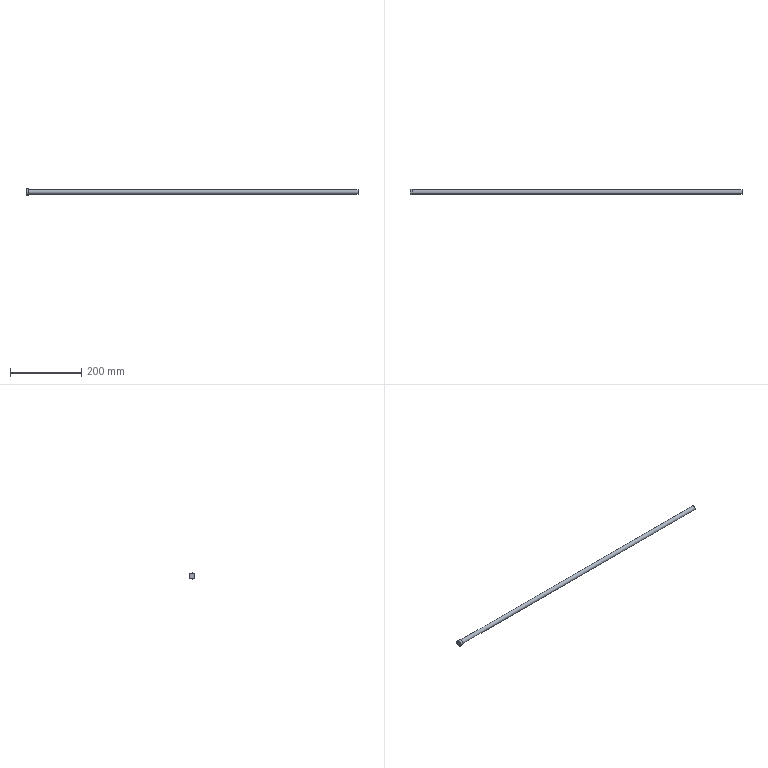Part | STEP file | solid 10 | 1 solid | 5 faces | box 935 x 17 x 17 mm | volume 106657 mm3 | plane 3 | cylinder 2 | commonest cylinder face diameters 12 x1 17 x1